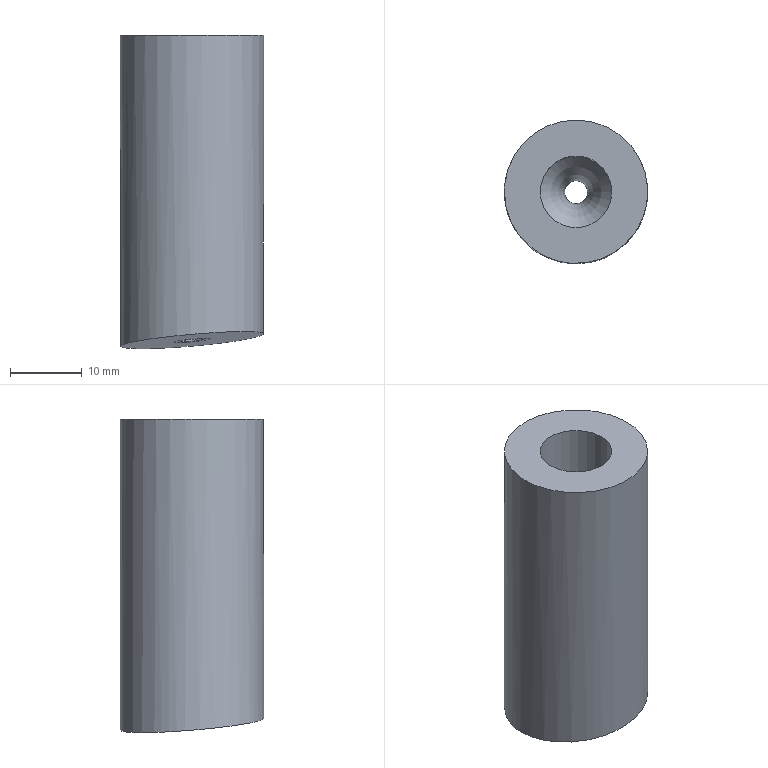Part | NX | features solid 2 | 1 solid | 7 faces | box 20 x 20 x 43.711 mm | volume 10716 mm3 | cylinder 3 | spline 2 | plane 1 | torus 1 | commonest cylinder face diameters 3.2 x1 10 x1 20 x1
STEP:
#1=CARTESIAN_POINT('',(507.735,-362.056,-35.));
#2=VERTEX_POINT('',#1);
#3=CARTESIAN_POINT('',(517.735,-362.056,-35.));
#4=DIRECTION('',(0.,0.,-1.));
#5=DIRECTION('',(-1.,0.,0.));
#6=AXIS2_PLACEMENT_3D('',#3,#4,#5);
#7=CIRCLE('',#6,10.);
#8=EDGE_CURVE('',#2,#2,#7,.T.);
#9=ORIENTED_EDGE('',*,*,#8,.F.);
#10=EDGE_LOOP('',(#9));
#11=FACE_BOUND('',#10,.T.);
#12=CARTESIAN_POINT('',(512.735,-362.056,-35.));
#13=VERTEX_POINT('',#12);
#14=CARTESIAN_POINT('',(517.735,-362.056,-35.));
#15=DIRECTION('',(0.,0.,-1.));
#16=DIRECTION('',(-1.,0.,0.));
#17=AXIS2_PLACEMENT_3D('',#14,#15,#16);
#18=CIRCLE('',#17,5.);
#19=EDGE_CURVE('',#13,#13,#18,.F.);
#20=ORIENTED_EDGE('',*,*,#19,.F.);
#21=EDGE_LOOP('',(#20));
#22=FACE_BOUND('',#21,.T.);
#23=CARTESIAN_POINT('',(517.735,-362.056,-35.));
#24=DIRECTION('',(0.,0.,-1.));
#25=DIRECTION('',(-1.,0.,0.));
#26=AXIS2_PLACEMENT_3D('',#23,#24,#25);
#27=PLANE('',#26);
#28=ADVANCED_FACE('',(#11,#22),#27,.F.);
#29=CARTESIAN_POINT('',(507.786,-361.053,-78.442));
#30=VERTEX_POINT('',#29);
#31=CARTESIAN_POINT('',(510.746,-353.439,-78.837));
#32=CARTESIAN_POINT('',(506.703,-360.956,-78.535));
#33=CARTESIAN_POINT('',(509.157,-369.054,-77.674));
#34=CARTESIAN_POINT('',(516.573,-373.072,-76.728));
#35=CARTESIAN_POINT('',(524.728,-370.669,-76.195));
#36=CARTESIAN_POINT('',(528.766,-363.154,-76.433));
#37=CARTESIAN_POINT('',(526.32,-355.07,-77.336));
#38=CARTESIAN_POINT('',(518.91,-351.039,-78.347));
#39=CARTESIAN_POINT('',(510.746,-353.439,-78.837));
#40=CARTESIAN_POINT('',(506.703,-360.956,-78.535));
#41=CARTESIAN_POINT('',(509.157,-369.054,-77.674));
#42=B_SPLINE_CURVE_WITH_KNOTS('',3,(#31,#32,#33,#34,#35,#36,#37,#38,#39,#40,#41),.UNSPECIFIED.,.T.,.F.,(1,1,1,1,1,1,1,1,1,1,1,1,1,1,1),(-0.02353,-0.01569,-0.007843,0.,0.007843,0.01569,0.02353,0.03137,0.03922,0.04706,0.0549,0.06274,0.07059,0.07843,0.08627),.UNSPECIFIED.);
#43=EDGE_CURVE('',#30,#30,#42,.T.);
#44=ORIENTED_EDGE('',*,*,#43,.T.);
#45=EDGE_LOOP('',(#44));
#46=FACE_BOUND('',#45,.T.);
#47=ORIENTED_EDGE('',*,*,#8,.T.);
#48=EDGE_LOOP('',(#47));
#49=FACE_BOUND('',#48,.T.);
#50=CARTESIAN_POINT('',(517.735,-362.056,-85.));
#51=DIRECTION('',(0.,0.,1.));
#52=DIRECTION('',(1.,0.,0.));
#53=AXIS2_PLACEMENT_3D('',#50,#51,#52);
#54=CYLINDRICAL_SURFACE('',#53,10.);
#55=ADVANCED_FACE('',(#46,#49),#54,.T.);
#56=CARTESIAN_POINT('',(512.735,-362.056,-65.705));
#57=VERTEX_POINT('',#56);
#58=CARTESIAN_POINT('',(517.735,-362.056,-65.705));
#59=DIRECTION('',(0.,0.,-1.));
#60=DIRECTION('',(-1.,0.,0.));
#61=AXIS2_PLACEMENT_3D('',#58,#59,#60);
#62=CIRCLE('',#61,5.);
#63=EDGE_CURVE('',#57,#57,#62,.F.);
#64=ORIENTED_EDGE('',*,*,#63,.F.);
#65=EDGE_LOOP('',(#64));
#66=FACE_BOUND('',#65,.T.);
#67=ORIENTED_EDGE('',*,*,#19,.T.);
#68=EDGE_LOOP('',(#67));
#69=FACE_BOUND('',#68,.T.);
#70=CARTESIAN_POINT('',(517.735,-362.056,-5.));
#71=DIRECTION('',(0.,0.,-1.));
#72=DIRECTION('',(0.,-1.,0.));
#73=AXIS2_PLACEMENT_3D('',#70,#71,#72);
#74=CYLINDRICAL_SURFACE('',#73,5.);
#75=ADVANCED_FACE('',(#66,#69),#74,.F.);
#76=CARTESIAN_POINT('',(517.735,-360.456,-77.674));
#77=VERTEX_POINT('',#76);
#78=CARTESIAN_POINT('',(516.477,-360.804,-77.754));
#79=CARTESIAN_POINT('',(517.738,-360.283,-77.688));
#80=CARTESIAN_POINT('',(518.986,-360.802,-77.536));
#81=CARTESIAN_POINT('',(519.508,-362.046,-77.387));
#82=CARTESIAN_POINT('',(518.994,-363.308,-77.328));
#83=CARTESIAN_POINT('',(517.734,-363.829,-77.395));
#84=CARTESIAN_POINT('',(516.487,-363.312,-77.546));
#85=CARTESIAN_POINT('',(515.962,-362.066,-77.694));
#86=CARTESIAN_POINT('',(516.477,-360.804,-77.754));
#87=CARTESIAN_POINT('',(517.738,-360.283,-77.688));
#88=CARTESIAN_POINT('',(518.986,-360.802,-77.536));
#89=B_SPLINE_CURVE_WITH_KNOTS('',3,(#78,#79,#80,#81,#82,#83,#84,#85,#86,#87,#88),.UNSPECIFIED.,.T.,.F.,(1,1,1,1,1,1,1,1,1,1,1,1,1,1,1),(-0.003765,-0.00251,-0.001255,0.,0.001255,0.00251,0.003765,0.005019,0.006274,0.007529,0.008784,0.01004,0.01129,0.01255,0.0138),.UNSPECIFIED.);
#90=EDGE_CURVE('',#77,#77,#89,.T.);
#91=ORIENTED_EDGE('',*,*,#90,.T.);
#92=EDGE_LOOP('',(#91));
#93=FACE_BOUND('',#92,.T.);
#94=CARTESIAN_POINT('',(519.335,-362.056,-73.614));
#95=VERTEX_POINT('',#94);
#96=CARTESIAN_POINT('',(517.735,-362.056,-73.614));
#97=DIRECTION('',(0.,0.,1.));
#98=DIRECTION('',(1.,0.,0.));
#99=AXIS2_PLACEMENT_3D('',#96,#97,#98);
#100=CIRCLE('',#99,1.6);
#101=EDGE_CURVE('',#95,#95,#100,.F.);
#102=ORIENTED_EDGE('',*,*,#101,.F.);
#103=EDGE_LOOP('',(#102));
#104=FACE_BOUND('',#103,.T.);
#105=CARTESIAN_POINT('',(517.735,-362.056,-95.));
#106=DIRECTION('',(0.,0.,1.));
#107=DIRECTION('',(0.,1.,0.));
#108=AXIS2_PLACEMENT_3D('',#105,#106,#107);
#109=CYLINDRICAL_SURFACE('',#108,1.6);
#110=ADVANCED_FACE('',(#93,#104),#109,.F.);
#111=ORIENTED_EDGE('',*,*,#101,.T.);
#112=EDGE_LOOP('',(#111));
#113=FACE_BOUND('',#112,.T.);
#114=ORIENTED_EDGE('',*,*,#63,.T.);
#115=EDGE_LOOP('',(#114));
#116=FACE_BOUND('',#115,.T.);
#117=CARTESIAN_POINT('',(517.735,-362.056,-73.614));
#118=DIRECTION('',(0.,0.,1.));
#119=DIRECTION('',(1.,0.,0.));
#120=AXIS2_PLACEMENT_3D('',#117,#118,#119);
#121=TOROIDAL_SURFACE('',#120,12.5,10.9);
#122=ADVANCED_FACE('',(#113,#116),#121,.T.);
#123=CARTESIAN_POINT('',(517.76,-359.566,-77.745));
#124=VERTEX_POINT('',#123);
#125=CARTESIAN_POINT('',(517.696,-364.549,-77.338));
#126=VERTEX_POINT('',#125);
#127=CARTESIAN_POINT('',(517.76,-359.566,-77.745));
#128=CARTESIAN_POINT('',(518.447,-359.57,-77.685));
#129=CARTESIAN_POINT('',(519.683,-360.111,-77.531));
#130=CARTESIAN_POINT('',(520.501,-362.079,-77.296));
#131=CARTESIAN_POINT('',(519.628,-364.028,-77.212));
#132=CARTESIAN_POINT('',(518.381,-364.553,-77.278));
#133=CARTESIAN_POINT('',(517.696,-364.549,-77.338));
#134=B_SPLINE_CURVE_WITH_KNOTS('',3,(#127,#128,#129,#130,#131,#132,#133),.UNSPECIFIED.,.F.,.F.,(4,1,1,1,4),(0.,0.25,0.5,0.75,1.),.UNSPECIFIED.);
#135=EDGE_CURVE('',#124,#126,#134,.T.);
#136=ORIENTED_EDGE('',*,*,#135,.F.);
#137=CARTESIAN_POINT('',(517.696,-364.549,-77.338));
#138=CARTESIAN_POINT('',(517.009,-364.545,-77.399));
#139=CARTESIAN_POINT('',(515.773,-364.004,-77.55));
#140=CARTESIAN_POINT('',(514.955,-362.035,-77.782));
#141=CARTESIAN_POINT('',(515.828,-360.087,-77.869));
#142=CARTESIAN_POINT('',(517.075,-359.562,-77.805));
#143=CARTESIAN_POINT('',(517.76,-359.566,-77.745));
#144=B_SPLINE_CURVE_WITH_KNOTS('',3,(#137,#138,#139,#140,#141,#142,#143),.UNSPECIFIED.,.F.,.F.,(4,1,1,1,4),(0.,0.25,0.5,0.75,1.),.UNSPECIFIED.);
#145=EDGE_CURVE('',#126,#124,#144,.T.);
#146=ORIENTED_EDGE('',*,*,#145,.F.);
#147=EDGE_LOOP('',(#136,#146));
#148=FACE_BOUND('',#147,.T.);
#149=ORIENTED_EDGE('',*,*,#43,.F.);
#150=EDGE_LOOP('',(#149));
#151=FACE_BOUND('',#150,.T.);
#152=CARTESIAN_POINT('',(507.607,-351.845,-79.203));
#153=CARTESIAN_POINT('',(511.684,-351.858,-78.888));
#154=CARTESIAN_POINT('',(515.759,-351.871,-78.553));
#155=CARTESIAN_POINT('',(519.832,-351.884,-78.198));
#156=CARTESIAN_POINT('',(523.902,-351.898,-77.822));
#157=CARTESIAN_POINT('',(527.969,-351.911,-77.426));
#158=CARTESIAN_POINT('',(507.607,-351.94,-79.196));
#159=CARTESIAN_POINT('',(511.684,-351.953,-78.881));
#160=CARTESIAN_POINT('',(515.759,-351.967,-78.546));
#161=CARTESIAN_POINT('',(519.831,-351.98,-78.19));
#162=CARTESIAN_POINT('',(523.901,-351.993,-77.815));
#163=CARTESIAN_POINT('',(527.969,-352.006,-77.418));
#164=CARTESIAN_POINT('',(507.606,-352.036,-79.188));
#165=CARTESIAN_POINT('',(511.683,-352.049,-78.873));
#166=CARTESIAN_POINT('',(515.758,-352.062,-78.538));
#167=CARTESIAN_POINT('',(519.831,-352.075,-78.183));
#168=CARTESIAN_POINT('',(523.901,-352.088,-77.807));
#169=CARTESIAN_POINT('',(527.968,-352.102,-77.411));
#170=CARTESIAN_POINT('',(507.606,-352.131,-79.18));
#171=CARTESIAN_POINT('',(511.683,-352.144,-78.866));
#172=CARTESIAN_POINT('',(515.758,-352.157,-78.531));
#173=CARTESIAN_POINT('',(519.83,-352.171,-78.175));
#174=CARTESIAN_POINT('',(523.9,-352.184,-77.799));
#175=CARTESIAN_POINT('',(527.968,-352.197,-77.403));
#176=CARTESIAN_POINT('',(507.605,-352.226,-79.173));
#177=CARTESIAN_POINT('',(511.682,-352.24,-78.858));
#178=CARTESIAN_POINT('',(515.757,-352.253,-78.523));
#179=CARTESIAN_POINT('',(519.83,-352.266,-78.167));
#180=CARTESIAN_POINT('',(523.9,-352.279,-77.792));
#181=CARTESIAN_POINT('',(527.967,-352.292,-77.396));
#182=CARTESIAN_POINT('',(507.605,-352.322,-79.165));
#183=CARTESIAN_POINT('',(511.682,-352.335,-78.85));
#184=CARTESIAN_POINT('',(515.757,-352.348,-78.515));
#185=CARTESIAN_POINT('',(519.829,-352.361,-78.16));
#186=CARTESIAN_POINT('',(523.899,-352.375,-77.784));
#187=CARTESIAN_POINT('',(527.967,-352.388,-77.388));
#188=CARTESIAN_POINT('',(507.584,-356.292,-78.849));
#189=CARTESIAN_POINT('',(511.661,-356.305,-78.534));
#190=CARTESIAN_POINT('',(515.736,-356.318,-78.199));
#191=CARTESIAN_POINT('',(519.808,-356.331,-77.843));
#192=CARTESIAN_POINT('',(523.878,-356.344,-77.467));
#193=CARTESIAN_POINT('',(527.945,-356.357,-77.071));
#194=CARTESIAN_POINT('',(507.563,-360.262,-78.527));
#195=CARTESIAN_POINT('',(511.64,-360.275,-78.212));
#196=CARTESIAN_POINT('',(515.714,-360.288,-77.877));
#197=CARTESIAN_POINT('',(519.786,-360.301,-77.522));
#198=CARTESIAN_POINT('',(523.856,-360.314,-77.146));
#199=CARTESIAN_POINT('',(527.923,-360.327,-76.75));
#200=CARTESIAN_POINT('',(507.541,-364.232,-78.2));
#201=CARTESIAN_POINT('',(511.618,-364.245,-77.886));
#202=CARTESIAN_POINT('',(515.692,-364.257,-77.55));
#203=CARTESIAN_POINT('',(519.764,-364.27,-77.195));
#204=CARTESIAN_POINT('',(523.834,-364.283,-76.819));
#205=CARTESIAN_POINT('',(527.901,-364.296,-76.423));
#206=CARTESIAN_POINT('',(507.519,-368.201,-77.869));
#207=CARTESIAN_POINT('',(511.596,-368.214,-77.554));
#208=CARTESIAN_POINT('',(515.67,-368.227,-77.219));
#209=CARTESIAN_POINT('',(519.742,-368.24,-76.863));
#210=CARTESIAN_POINT('',(523.811,-368.252,-76.488));
#211=CARTESIAN_POINT('',(527.878,-368.265,-76.091));
#212=CARTESIAN_POINT('',(507.497,-372.171,-77.532));
#213=CARTESIAN_POINT('',(511.573,-372.183,-77.217));
#214=CARTESIAN_POINT('',(515.647,-372.196,-76.882));
#215=CARTESIAN_POINT('',(519.719,-372.209,-76.527));
#216=CARTESIAN_POINT('',(523.788,-372.221,-76.151));
#217=CARTESIAN_POINT('',(527.855,-372.234,-75.755));
#218=B_SPLINE_SURFACE_WITH_KNOTS('',5,5,((#152,#153,#154,#155,#156,#157),(#158,#159,#160,#161,#162,#163),(#164,#165,#166,#167,#168,#169),(#170,#171,#172,#173,#174,#175),(#176,#177,#178,#179,#180,#181),(#182,#183,#184,#185,#186,#187),(#188,#189,#190,#191,#192,#193),(#194,#195,#196,#197,#198,#199),(#200,#201,#202,#203,#204,#205),(#206,#207,#208,#209,#210,#211),(#212,#213,#214,#215,#216,#217)),.UNSPECIFIED.,.F.,.F.,.F.,(6,5,6),(6,6),(-0.01936,0.,0.8058),(0.2584,0.7186),.PIECEWISE_BEZIER_KNOTS.);
#219=ADVANCED_FACE('',(#148,#151),#218,.F.);
#220=ORIENTED_EDGE('',*,*,#145,.T.);
#221=ORIENTED_EDGE('',*,*,#135,.T.);
#222=EDGE_LOOP('',(#220,#221));
#223=FACE_BOUND('',#222,.T.);
#224=ORIENTED_EDGE('',*,*,#90,.F.);
#225=EDGE_LOOP('',(#224));
#226=FACE_BOUND('',#225,.T.);
#227=CARTESIAN_POINT('',(515.211,-359.525,-77.967));
#228=CARTESIAN_POINT('',(516.223,-359.528,-77.881));
#229=CARTESIAN_POINT('',(517.234,-359.532,-77.794));
#230=CARTESIAN_POINT('',(518.245,-359.535,-77.706));
#231=CARTESIAN_POINT('',(519.257,-359.538,-77.616));
#232=CARTESIAN_POINT('',(520.268,-359.541,-77.526));
#233=CARTESIAN_POINT('',(515.206,-360.535,-77.885));
#234=CARTESIAN_POINT('',(516.217,-360.538,-77.799));
#235=CARTESIAN_POINT('',(517.229,-360.541,-77.712));
#236=CARTESIAN_POINT('',(518.24,-360.544,-77.624));
#237=CARTESIAN_POINT('',(519.251,-360.547,-77.534));
#238=CARTESIAN_POINT('',(520.262,-360.551,-77.443));
#239=CARTESIAN_POINT('',(515.2,-361.544,-77.802));
#240=CARTESIAN_POINT('',(516.212,-361.547,-77.716));
#241=CARTESIAN_POINT('',(517.223,-361.551,-77.629));
#242=CARTESIAN_POINT('',(518.234,-361.554,-77.541));
#243=CARTESIAN_POINT('',(519.245,-361.557,-77.451));
#244=CARTESIAN_POINT('',(520.256,-361.56,-77.361));
#245=CARTESIAN_POINT('',(515.194,-362.554,-77.719));
#246=CARTESIAN_POINT('',(516.206,-362.557,-77.633));
#247=CARTESIAN_POINT('',(517.217,-362.56,-77.546));
#248=CARTESIAN_POINT('',(518.229,-362.563,-77.458));
#249=CARTESIAN_POINT('',(519.24,-362.566,-77.368));
#250=CARTESIAN_POINT('',(520.251,-362.57,-77.278));
#251=CARTESIAN_POINT('',(515.189,-363.563,-77.636));
#252=CARTESIAN_POINT('',(516.2,-363.566,-77.55));
#253=CARTESIAN_POINT('',(517.212,-363.569,-77.463));
#254=CARTESIAN_POINT('',(518.223,-363.573,-77.375));
#255=CARTESIAN_POINT('',(519.234,-363.576,-77.285));
#256=CARTESIAN_POINT('',(520.245,-363.579,-77.194));
#257=CARTESIAN_POINT('',(515.183,-364.572,-77.552));
#258=CARTESIAN_POINT('',(516.195,-364.576,-77.466));
#259=CARTESIAN_POINT('',(517.206,-364.579,-77.379));
#260=CARTESIAN_POINT('',(518.218,-364.582,-77.291));
#261=CARTESIAN_POINT('',(519.229,-364.585,-77.201));
#262=CARTESIAN_POINT('',(520.24,-364.588,-77.111));
#263=B_SPLINE_SURFACE_WITH_KNOTS('',5,5,((#227,#228,#229,#230,#231,#232),(#233,#234,#235,#236,#237,#238),(#239,#240,#241,#242,#243,#244),(#245,#246,#247,#248,#249,#250),(#251,#252,#253,#254,#255,#256),(#257,#258,#259,#260,#261,#262)),.UNSPECIFIED.,.F.,.F.,.F.,(6,6),(6,6),(0.2914,0.4964),(0.431,0.5453),.PIECEWISE_BEZIER_KNOTS.);
#264=ADVANCED_FACE('',(#223,#226),#263,.F.);
#265=CLOSED_SHELL('',(#28,#55,#75,#110,#122,#219,#264));
#266=MANIFOLD_SOLID_BREP('',#265);
#267=(LENGTH_UNIT()NAMED_UNIT(*)SI_UNIT(.MILLI.,.METRE.));
#268=UNCERTAINTY_MEASURE_WITH_UNIT(LENGTH_MEASURE(0.0508),#267,'','');
#269=(NAMED_UNIT(*)PLANE_ANGLE_UNIT()SI_UNIT($,.RADIAN.));
#270=(NAMED_UNIT(*)SI_UNIT($,.STERADIAN.)SOLID_ANGLE_UNIT());
#271=(GEOMETRIC_REPRESENTATION_CONTEXT(3)GLOBAL_UNCERTAINTY_ASSIGNED_CONTEXT((#268))GLOBAL_UNIT_ASSIGNED_CONTEXT((#267,#269,#270))REPRESENTATION_CONTEXT('',''));
#272=ADVANCED_BREP_SHAPE_REPRESENTATION('',(#266),#271);